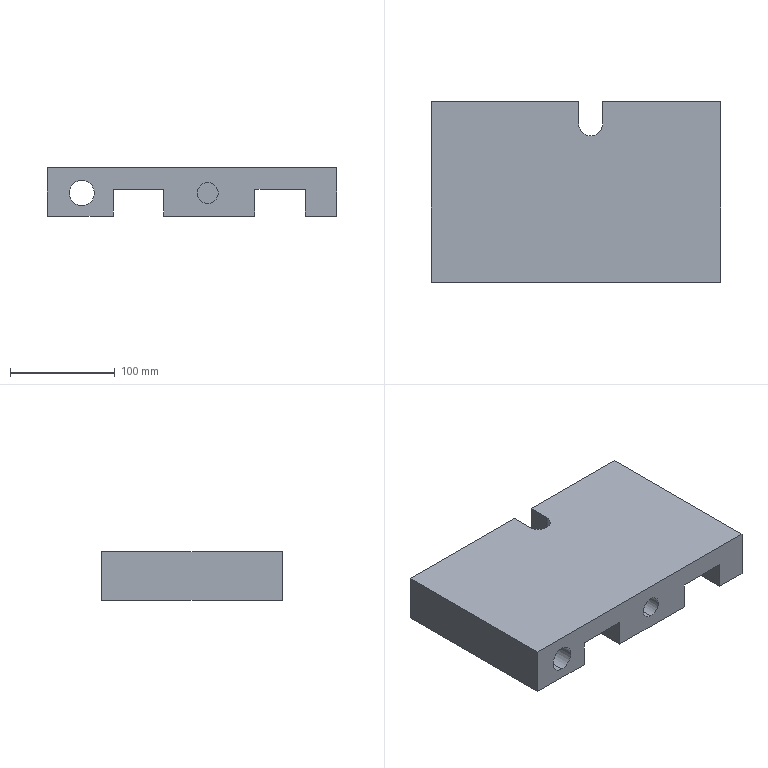Part | 1 solid | 23 faces | box 275.4 x 172 x 46 mm | volume 1638899 mm3 | plane 18 | cylinder 5 | commonest cylinder face diameters 20 x2 24 x2 23 x1